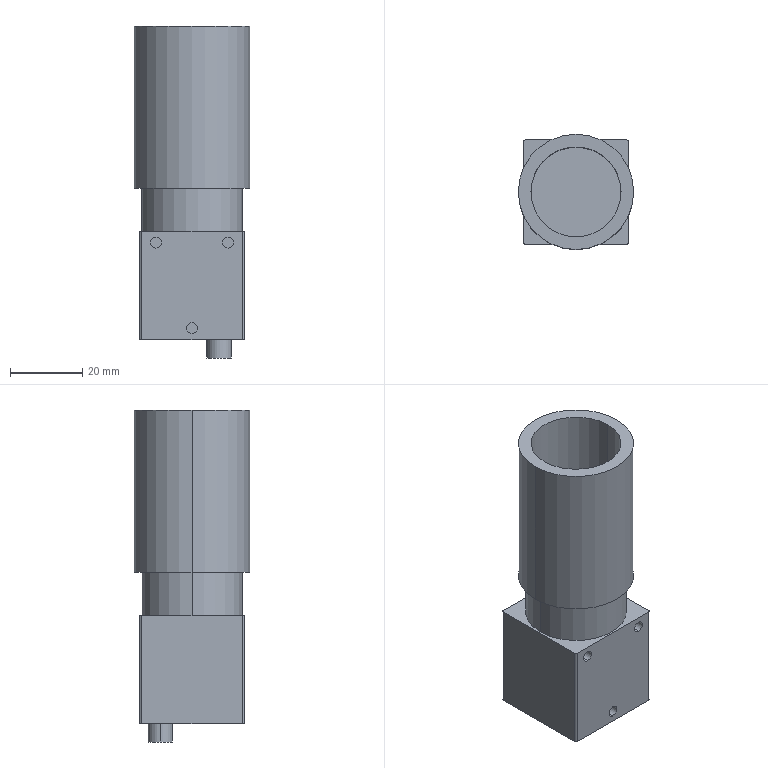Part | STEP file | ASND-0110-PG Flea2-1 | 1 solid | 31 faces | box 32 x 32 x 92.1 mm | volume 40913 mm3 | cylinder 18 | plane 13 | commonest cylinder face diameters 3 x6 1 x4 6.822 x2 25 x2 28 x2 32 x2